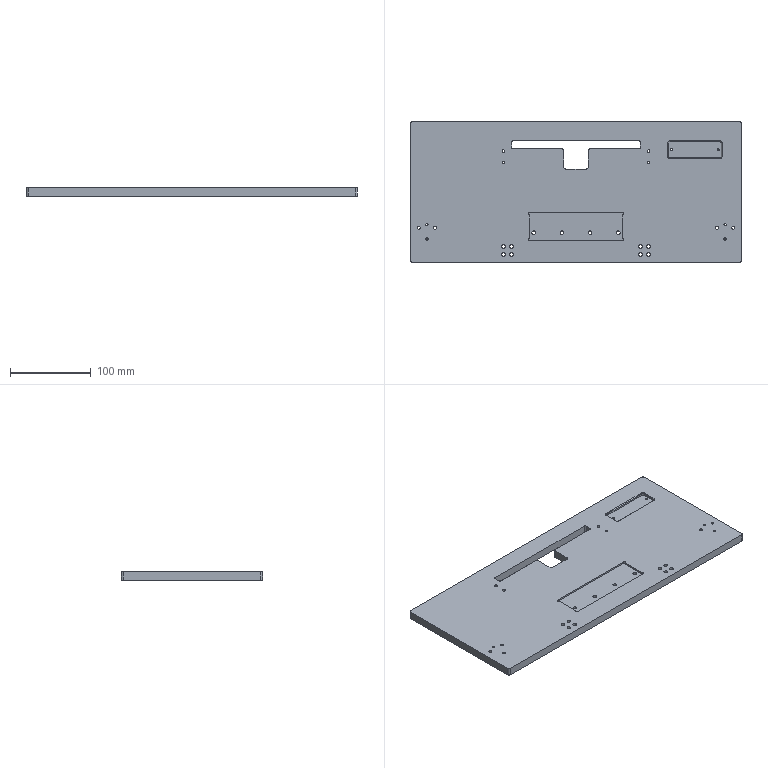Part | 1 solid | 140 faces | box 410 x 175 x 10 mm | volume 676501 mm3 | cylinder 96 | plane 40 | cone 4 | commonest cylinder face diameters 4.5 x24 3.5 x16 8.5 x16 3 x12 4 x12 8 x8